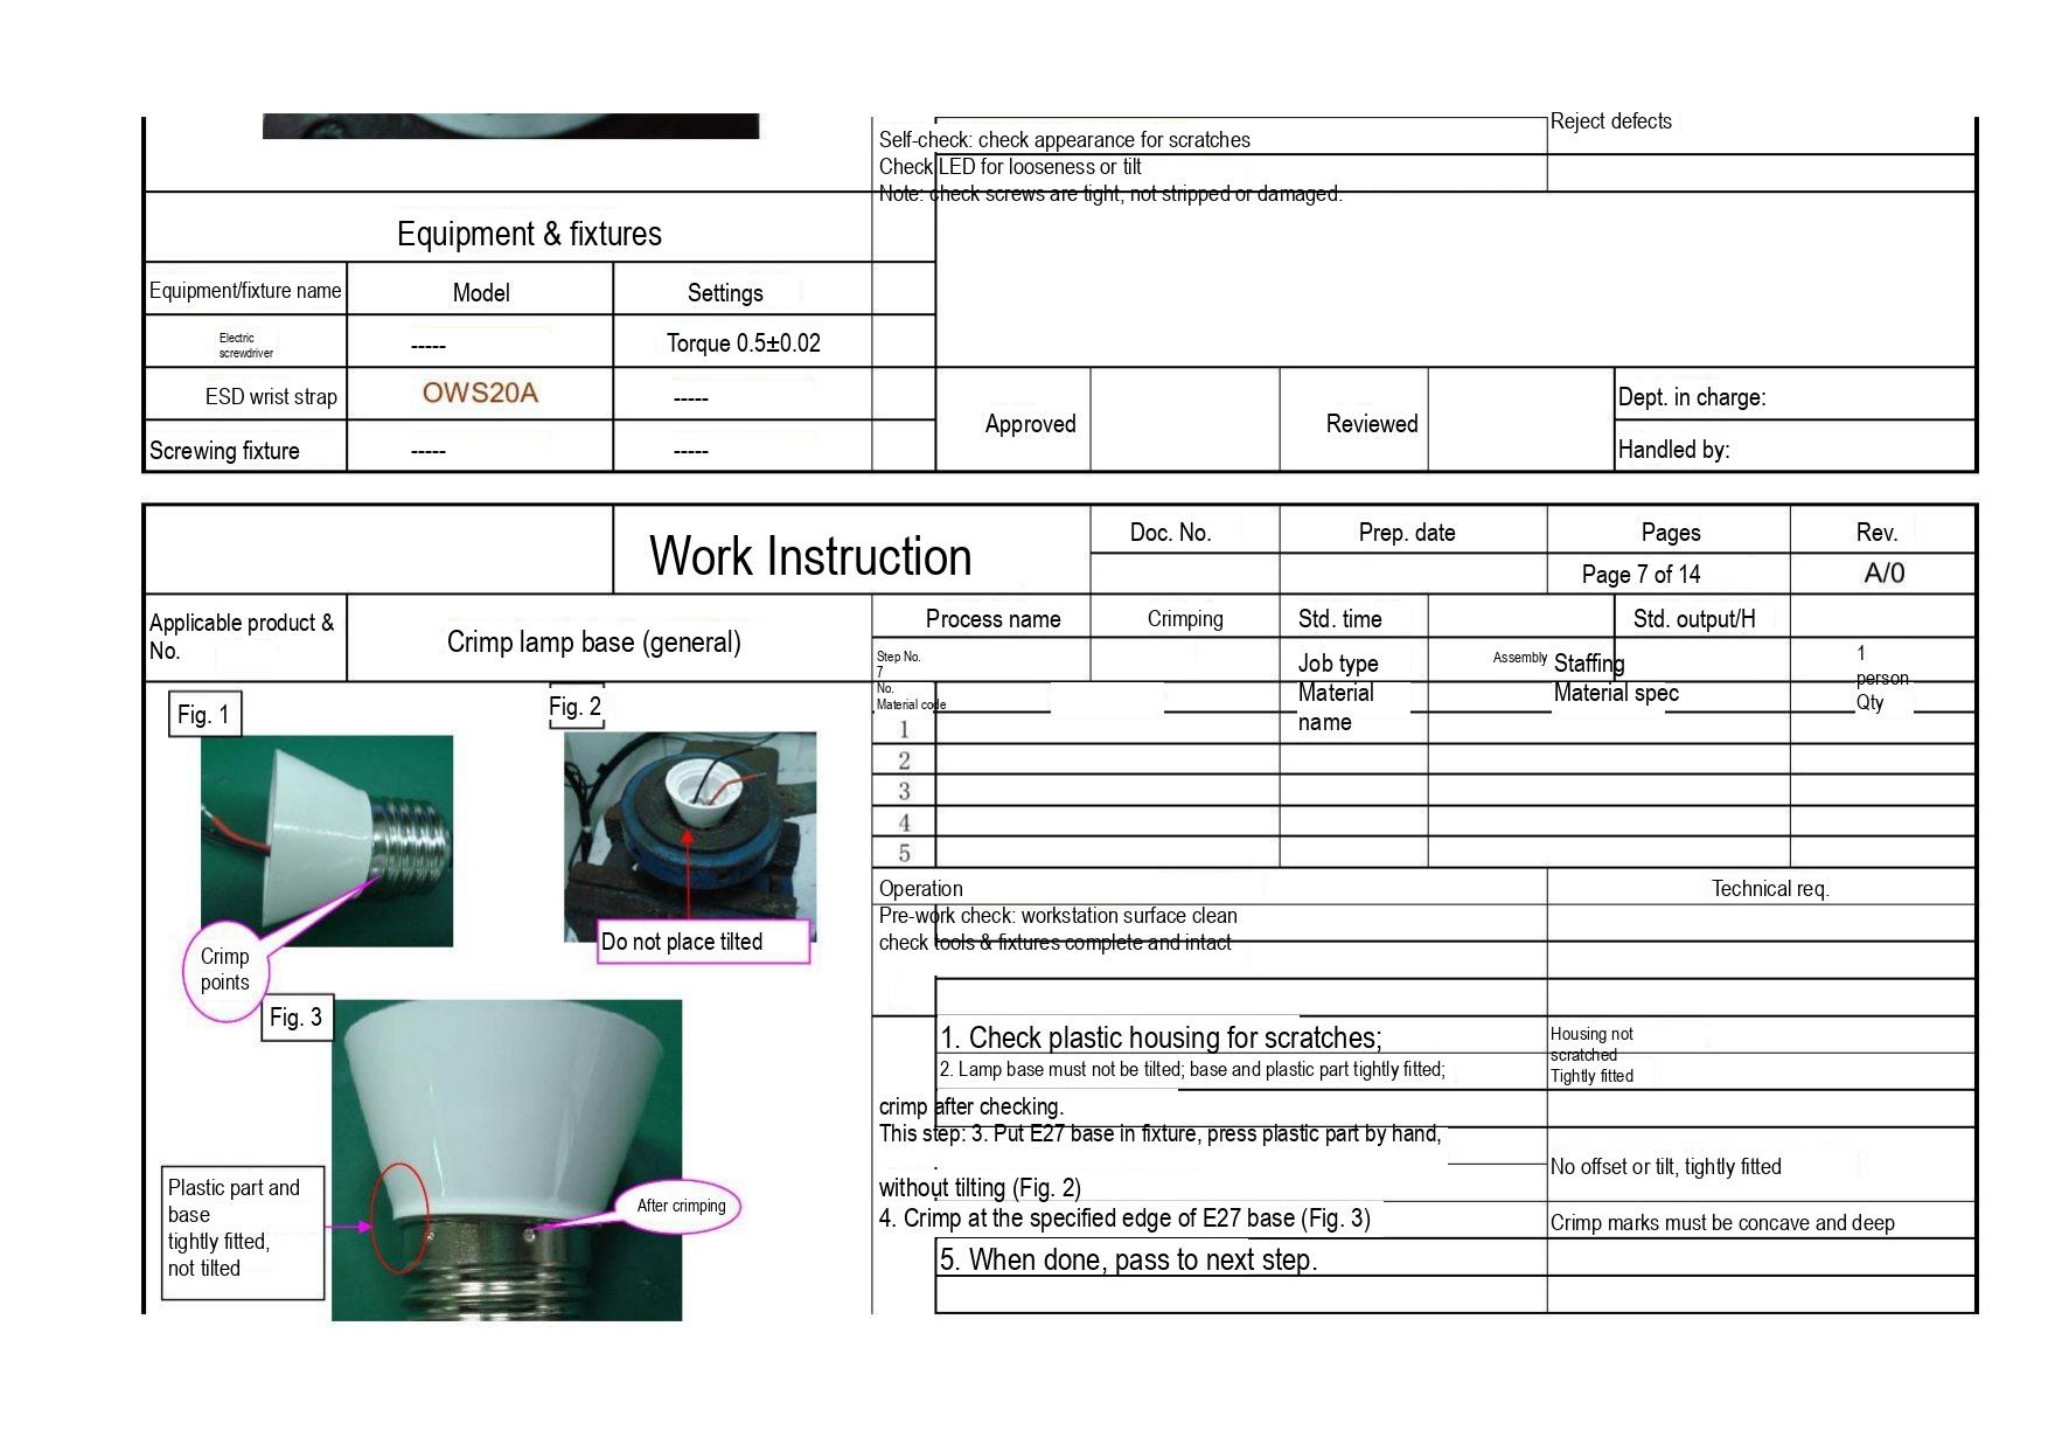Self-check: check appearance for scratches | Reject defects
Check LED for looseness or tilt
Note: check screws are tight, not stripped or damaged.

Equipment & fixtures

| Equipment/fixture name | Model | Settings |
|---|---|---|
| Electric screwdriver | ----- | Torque 0.5±0.02 |
| ESD wrist strap | OWS20A | ----- |
| Screwing fixture | ----- | ----- |

| Approved | | Reviewed | | Dept. in charge: |
|---|---|---|---|---|
| | | | | Handled by: |

| | Work Instruction | Doc. No. | Prep. date | Pages | Rev. |
|---|---|---|---|---|---|
| | | | | Page 7 of 14 | A/0 |

| Applicable product & No. | Crimp lamp base (general) |
|---|---|

| Process name | Crimping | Std. time | | Std. output/H | |
|---|---|---|---|---|---|
| Step No. 7 | | Job type | Assembly | Staffing | 1 person |
| No. | Material code | Material name | | Material spec | Qty |
| 1 | | | | | |
| 2 | | | | | |
| 3 | | | | | |
| 4 | | | | | |
| 5 | | | | | |

Fig. 1
Crimp points

Fig. 2
Do not place tilted

Fig. 3
Plastic part and base tightly fitted, not tilted
After crimping

| Operation | Technical req. |
|---|---|
| Pre-work check: workstation surface clean | |
| check tools & fixtures complete and intact | |
| 1. Check plastic housing for scratches; | Housing not scratched |
| 2. Lamp base must not be tilted; base and plastic part tightly fitted; | Tightly fitted |
| crimp after checking. | |
| This step: 3. Put E27 base in fixture, press plastic part by hand, without tilting (Fig. 2) | No offset or tilt, tightly fitted |
| 4. Crimp at the specified edge of E27 base (Fig. 3) | Crimp marks must be concave and deep |
| 5. When done, pass to next step. | |
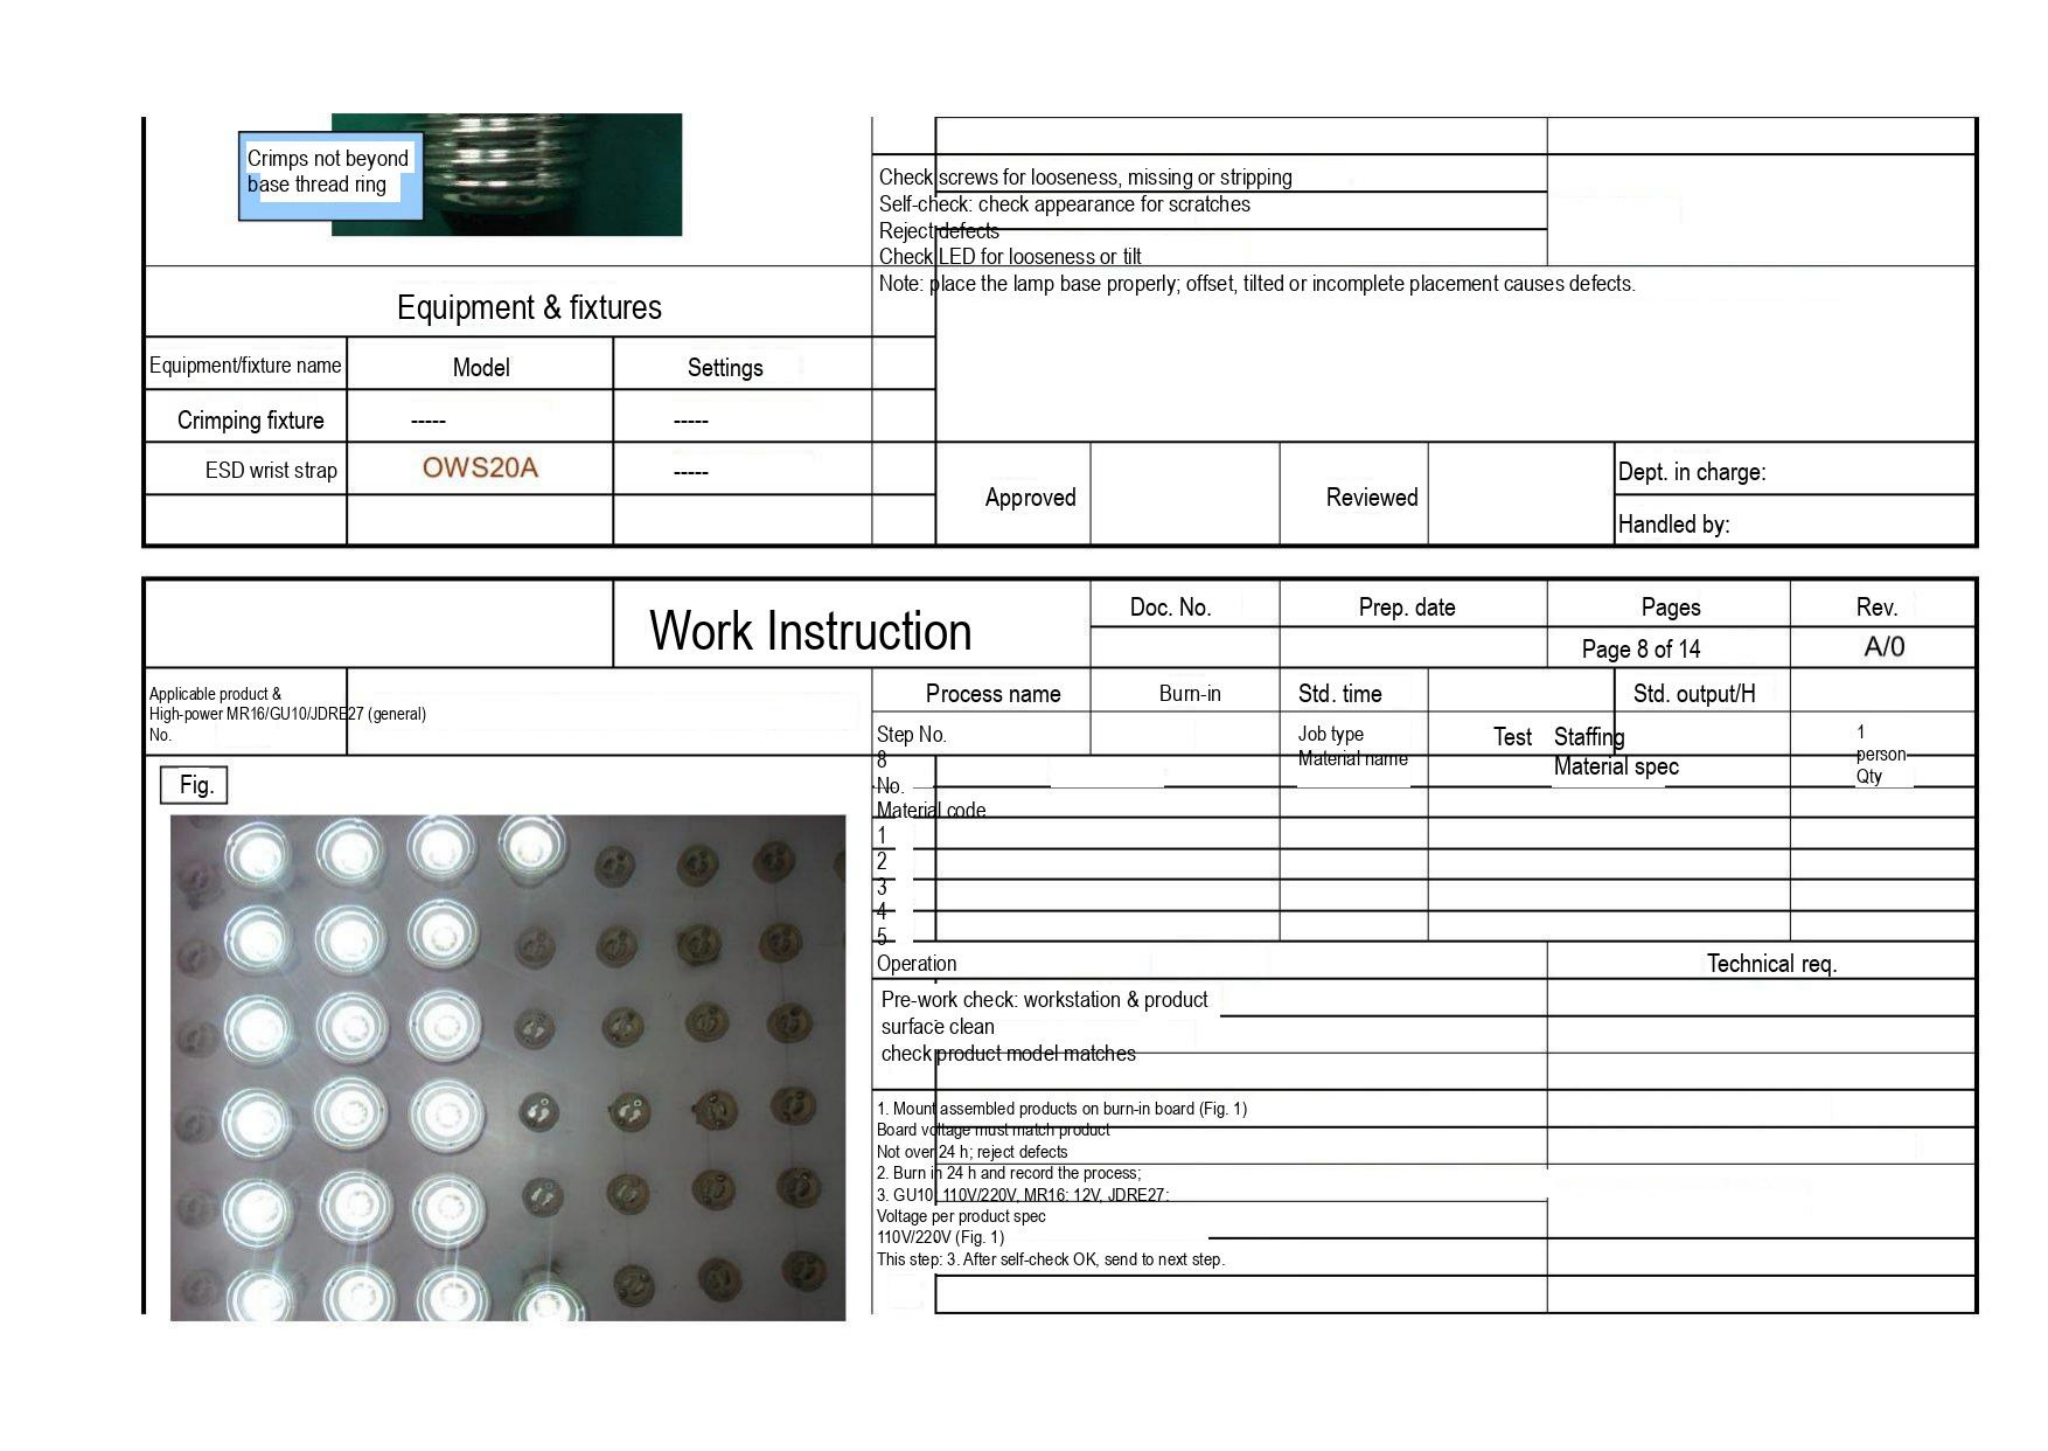Crimps not beyond base thread ring

Check screws for looseness, missing or stripping
Self-check: check appearance for scratches
Reject defects
Check LED for looseness or tilt
Note: place the lamp base properly; offset, tilted or incomplete placement causes defects.

Equipment & fixtures

| Equipment/fixture name | Model | Settings |
|---|---|---|
| Crimping fixture | ----- | ----- |
| ESD wrist strap | OWS20A | ----- |
| | | |

| Approved | | Reviewed | | Dept. in charge: |
|---|---|---|---|---|
| | | | | Handled by: |

| | Work Instruction | Doc. No. | Prep. date | Pages | Rev. |
|---|---|---|---|---|---|
| | | | | Page 8 of 14 | A/0 |

Applicable product & No. High-power MR16/GU10/JDRE27 (general)

| Process name | Burn-in | Std. time | | Std. output/H | |
|---|---|---|---|---|---|
| Step No. 8 | | Job type | Test | Staffing | 1 person |

| No. | Material code | Material name | Material spec | Qty |
|---|---|---|---|---|
| 1 | | | | |
| 2 | | | | |
| 3 | | | | |
| 4 | | | | |
| 5 | | | | |

Fig.

| Operation | Technical req. |
|---|---|
| Pre-work check: workstation & product surface clean check product model matches | |
| 1. Mount assembled products on burn-in board (Fig. 1) Board voltage must match product Not over 24 h; reject defects 2. Burn in 24 h and record the process; 3. GU10 110V/220V, MR16: 12V, JDRE27: Voltage per product spec 110V/220V (Fig. 1) This step: 3. After self-check OK, send to next step. | |
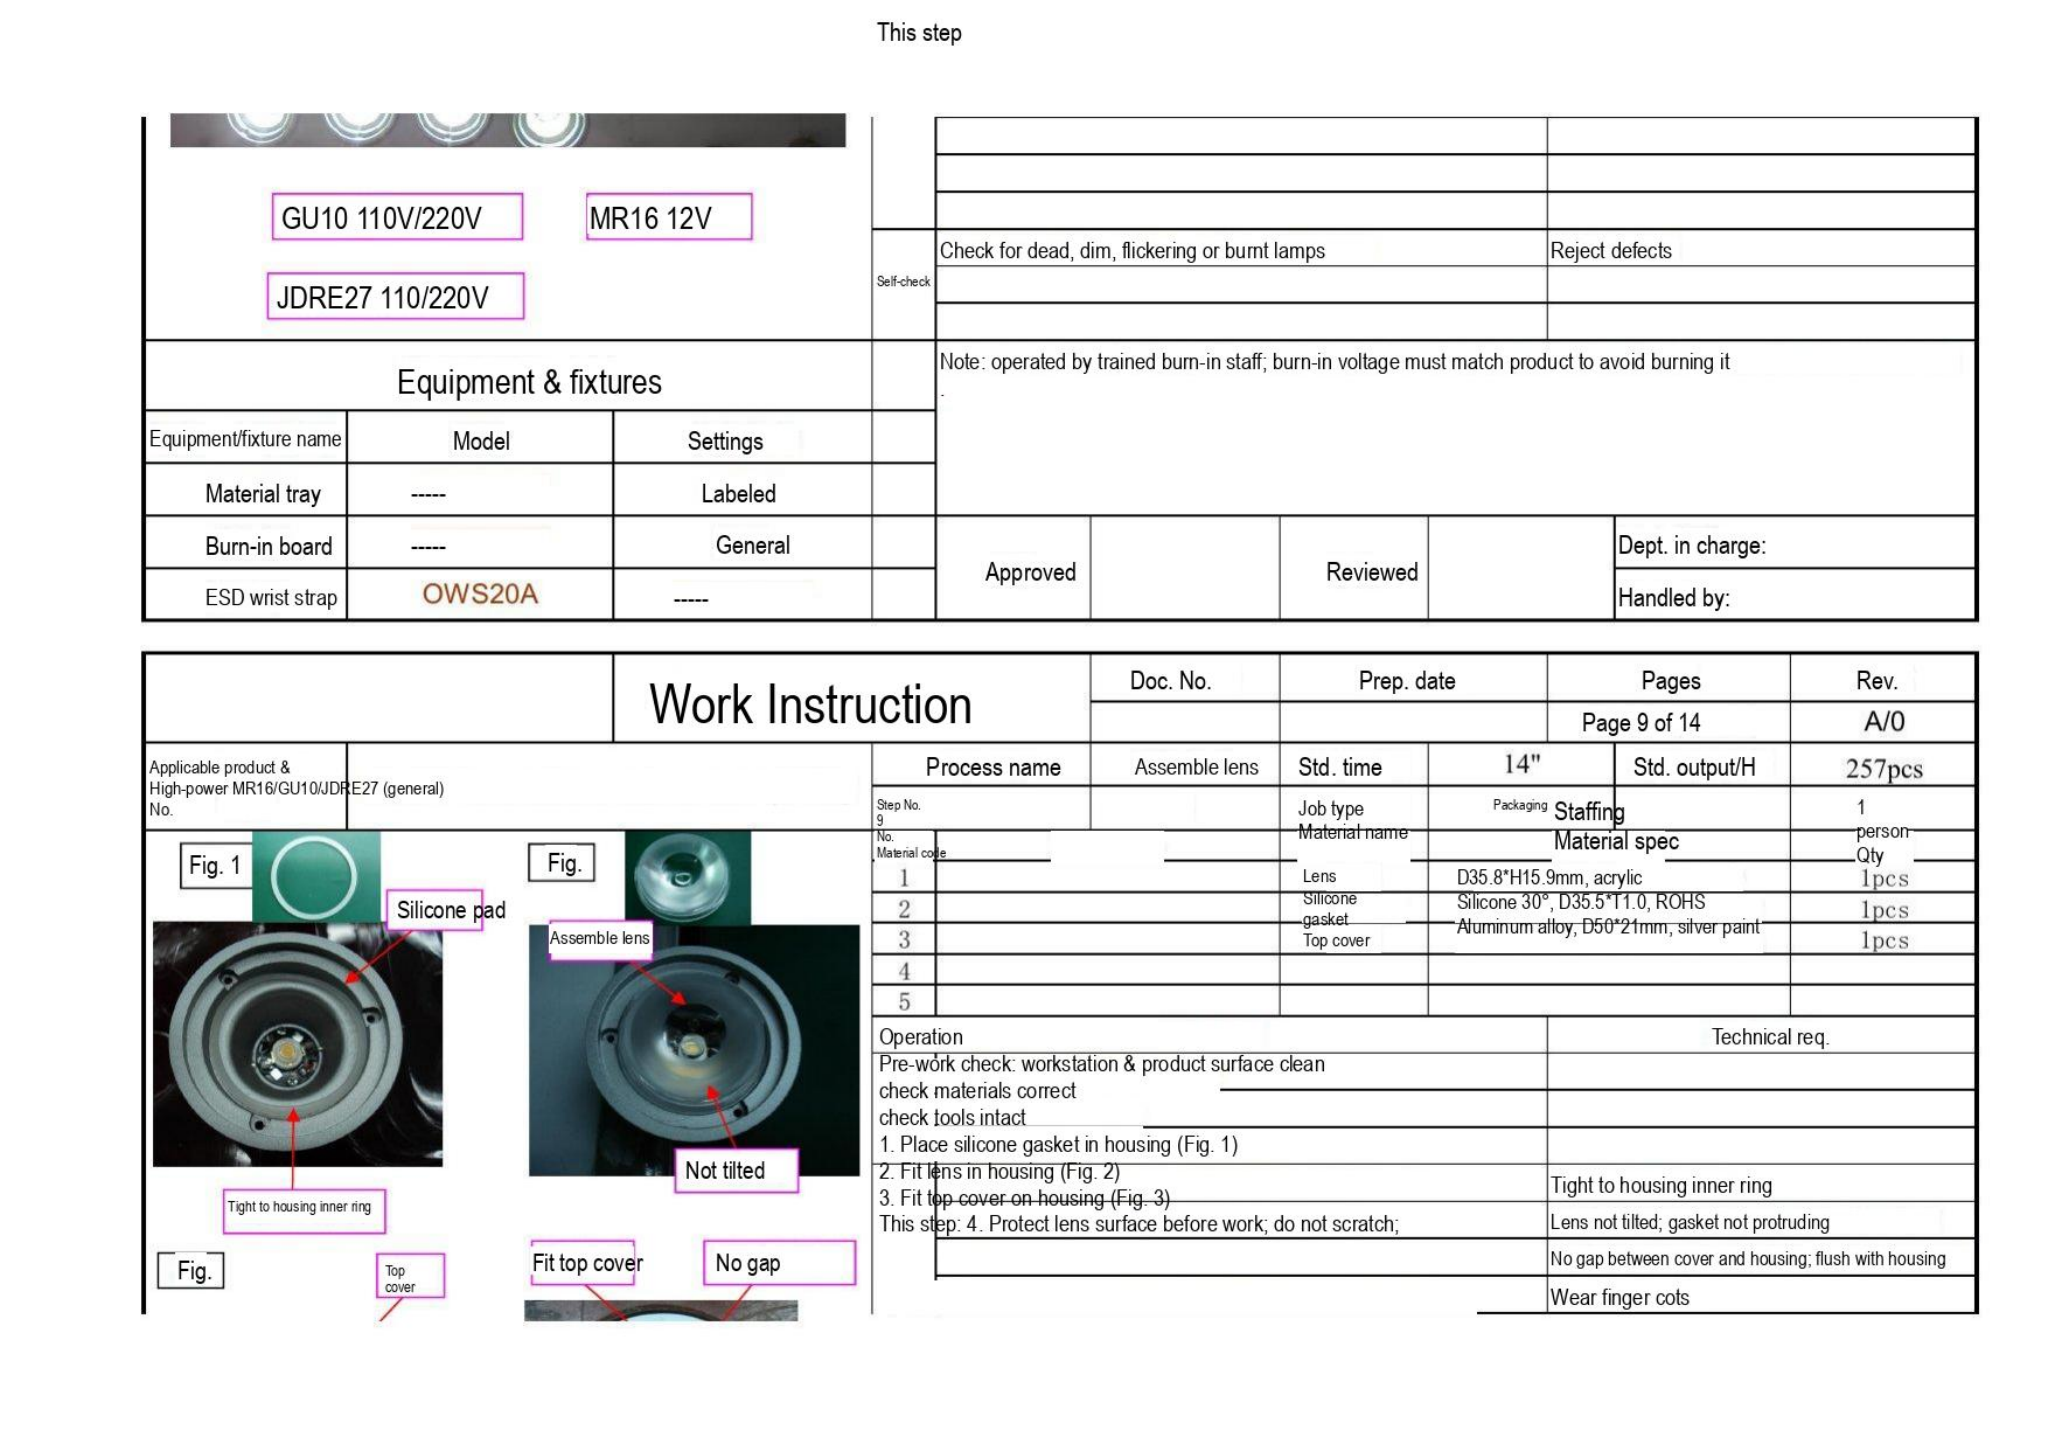This step

GU10 110V/220V

MR16 12V

JDRE27 110/220V

| Self-check | | |
|---|---|---|
| | | |
| | | |
| | | |
| | Check for dead, dim, flickering or burnt lamps | Reject defects |
| | | |
| | | |

Note: operated by trained burn-in staff; burn-in voltage must match product to avoid burning it

**Equipment & fixtures**

| Equipment/fixture name | Model | Settings |
|---|---|---|
| Material tray | ----- | Labeled |
| Burn-in board | ----- | General |
| ESD wrist strap | OWS20A | ----- |

| Approved | | Reviewed | | Dept. in charge: |
|---|---|---|---|---|
| | | | | Handled by: |

**Work Instruction**

| Doc. No. | Prep. date | Pages | Rev. |
|---|---|---|---|
| | | Page 9 of 14 | A/0 |

Applicable product & High-power MR16/GU10/JDRE27 (general)
No.

| Process name | Assemble lens | Std. time | 14" | Std. output/H | 257pcs |
|---|---|---|---|---|---|
| Step No. 9 | | Job type | Packaging | Staffing | 1 person |

| No. | Material code | Material name | Material spec | Qty |
|---|---|---|---|---|
| 1 | | Lens | D35.8*H15.9mm, acrylic | 1pcs |
| 2 | | Silicone gasket | Silicone 30°, D35.5*T1.0, ROHS | 1pcs |
| 3 | | Top cover | Aluminum alloy, D50*21mm, silver paint | 1pcs |
| 4 | | | | |
| 5 | | | | |

| Operation | Technical req. |
|---|---|
| Pre-work check: workstation & product surface clean | |
| check materials correct | |
| check tools intact | |
| 1. Place silicone gasket in housing (Fig. 1) | |
| 2. Fit lens in housing (Fig. 2) | Tight to housing inner ring |
| 3. Fit top cover on housing (Fig. 3) | Lens not tilted; gasket not protruding |
| This step: 4. Protect lens surface before work; do not scratch; | No gap between cover and housing; flush with housing |
| | Wear finger cots |

Fig. 1

Silicone pad

Tight to housing inner ring

Fig.

Assemble lens

Not tilted

Fig.

Top cover

Fit top cover

No gap
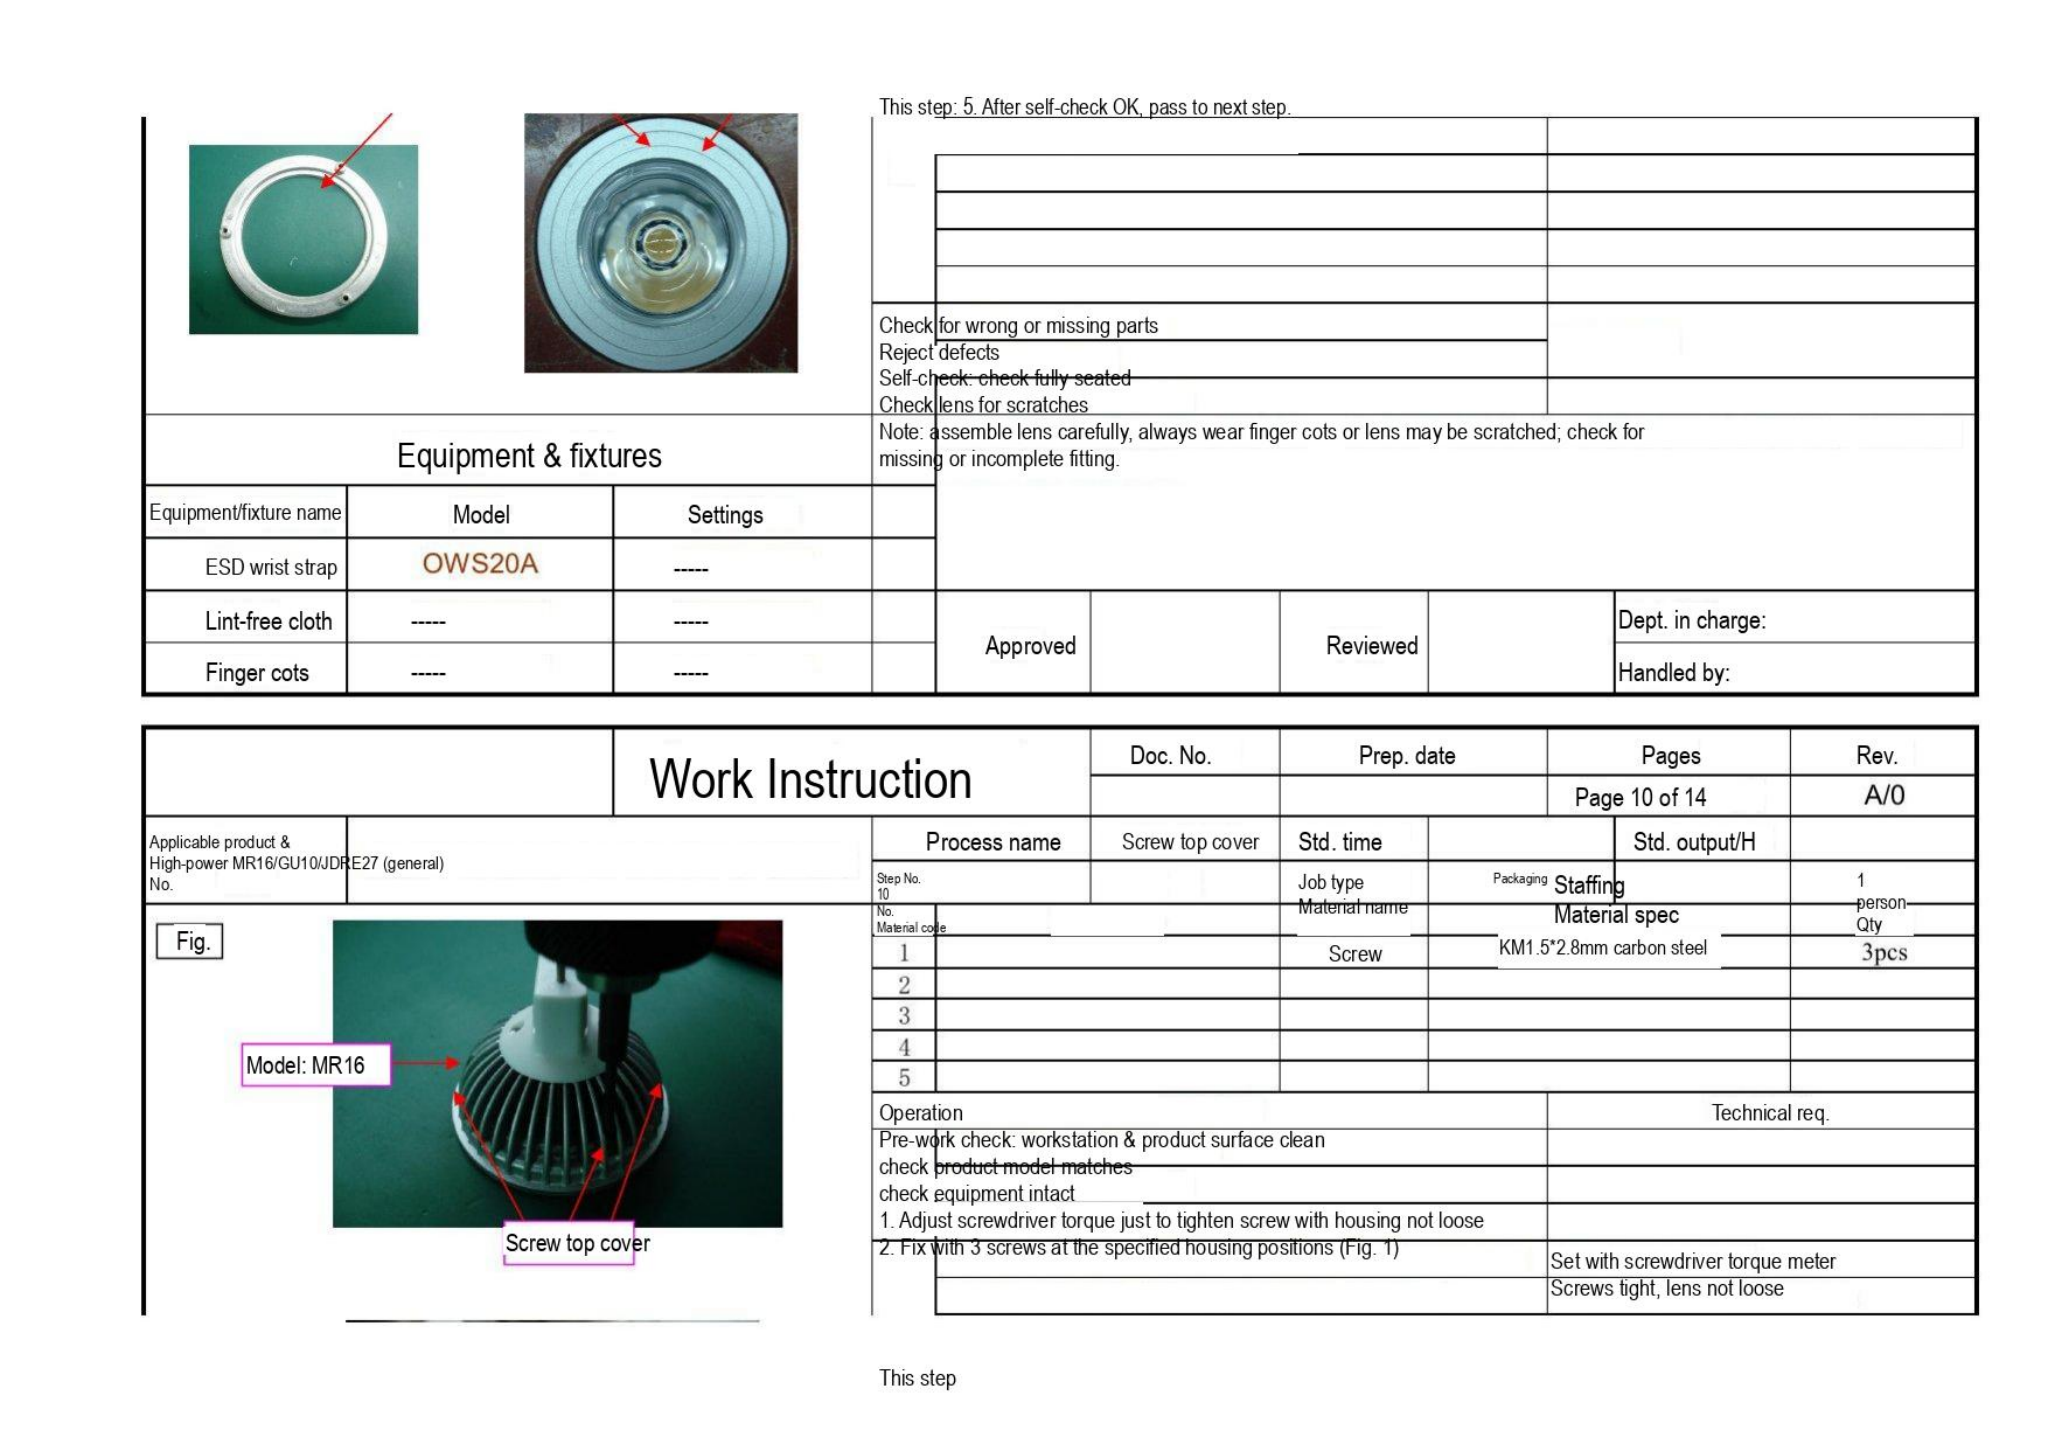This step: 5. After self-check OK, pass to next step.

Check for wrong or missing parts
Reject defects
Self-check: check fully seated
Check lens for scratches
Note: assemble lens carefully, always wear finger cots or lens may be scratched; check for missing or incomplete fitting.

Equipment & fixtures

| Equipment/fixture name | Model | Settings |
|---|---|---|
| ESD wrist strap | OWS20A | ----- |
| Lint-free cloth | ----- | ----- |
| Finger cots | ----- | ----- |

| Approved | | Reviewed | | Dept. in charge: |
|---|---|---|---|---|
| | | | | Handled by: |

Work Instruction

| Doc. No. | Prep. date | Pages | Rev. |
|---|---|---|---|
| | | Page 10 of 14 | A/0 |

Applicable product &
High-power MR16/GU10/JDRE27 (general)
No.

| Process name | Screw top cover | Std. time | | Std. output/H | |
|---|---|---|---|---|---|
| Step No. 10 | | Job type | Packaging | Staffing | 1 person |

| No. | Material code | Material name | Material spec | Qty |
|---|---|---|---|---|
| 1 | | Screw | KM1.5*2.8mm carbon steel | 3pcs |
| 2 | | | | |
| 3 | | | | |
| 4 | | | | |
| 5 | | | | |

Fig.

Model: MR16

Screw top cover

| Operation | Technical req. |
|---|---|
| Pre-work check: workstation & product surface clean | |
| check product model matches | |
| check equipment intact | |
| 1. Adjust screwdriver torque just to tighten screw with housing not loose | Set with screwdriver torque meter |
| 2. Fix with 3 screws at the specified housing positions (Fig. 1) | Screws tight, lens not loose |

This step
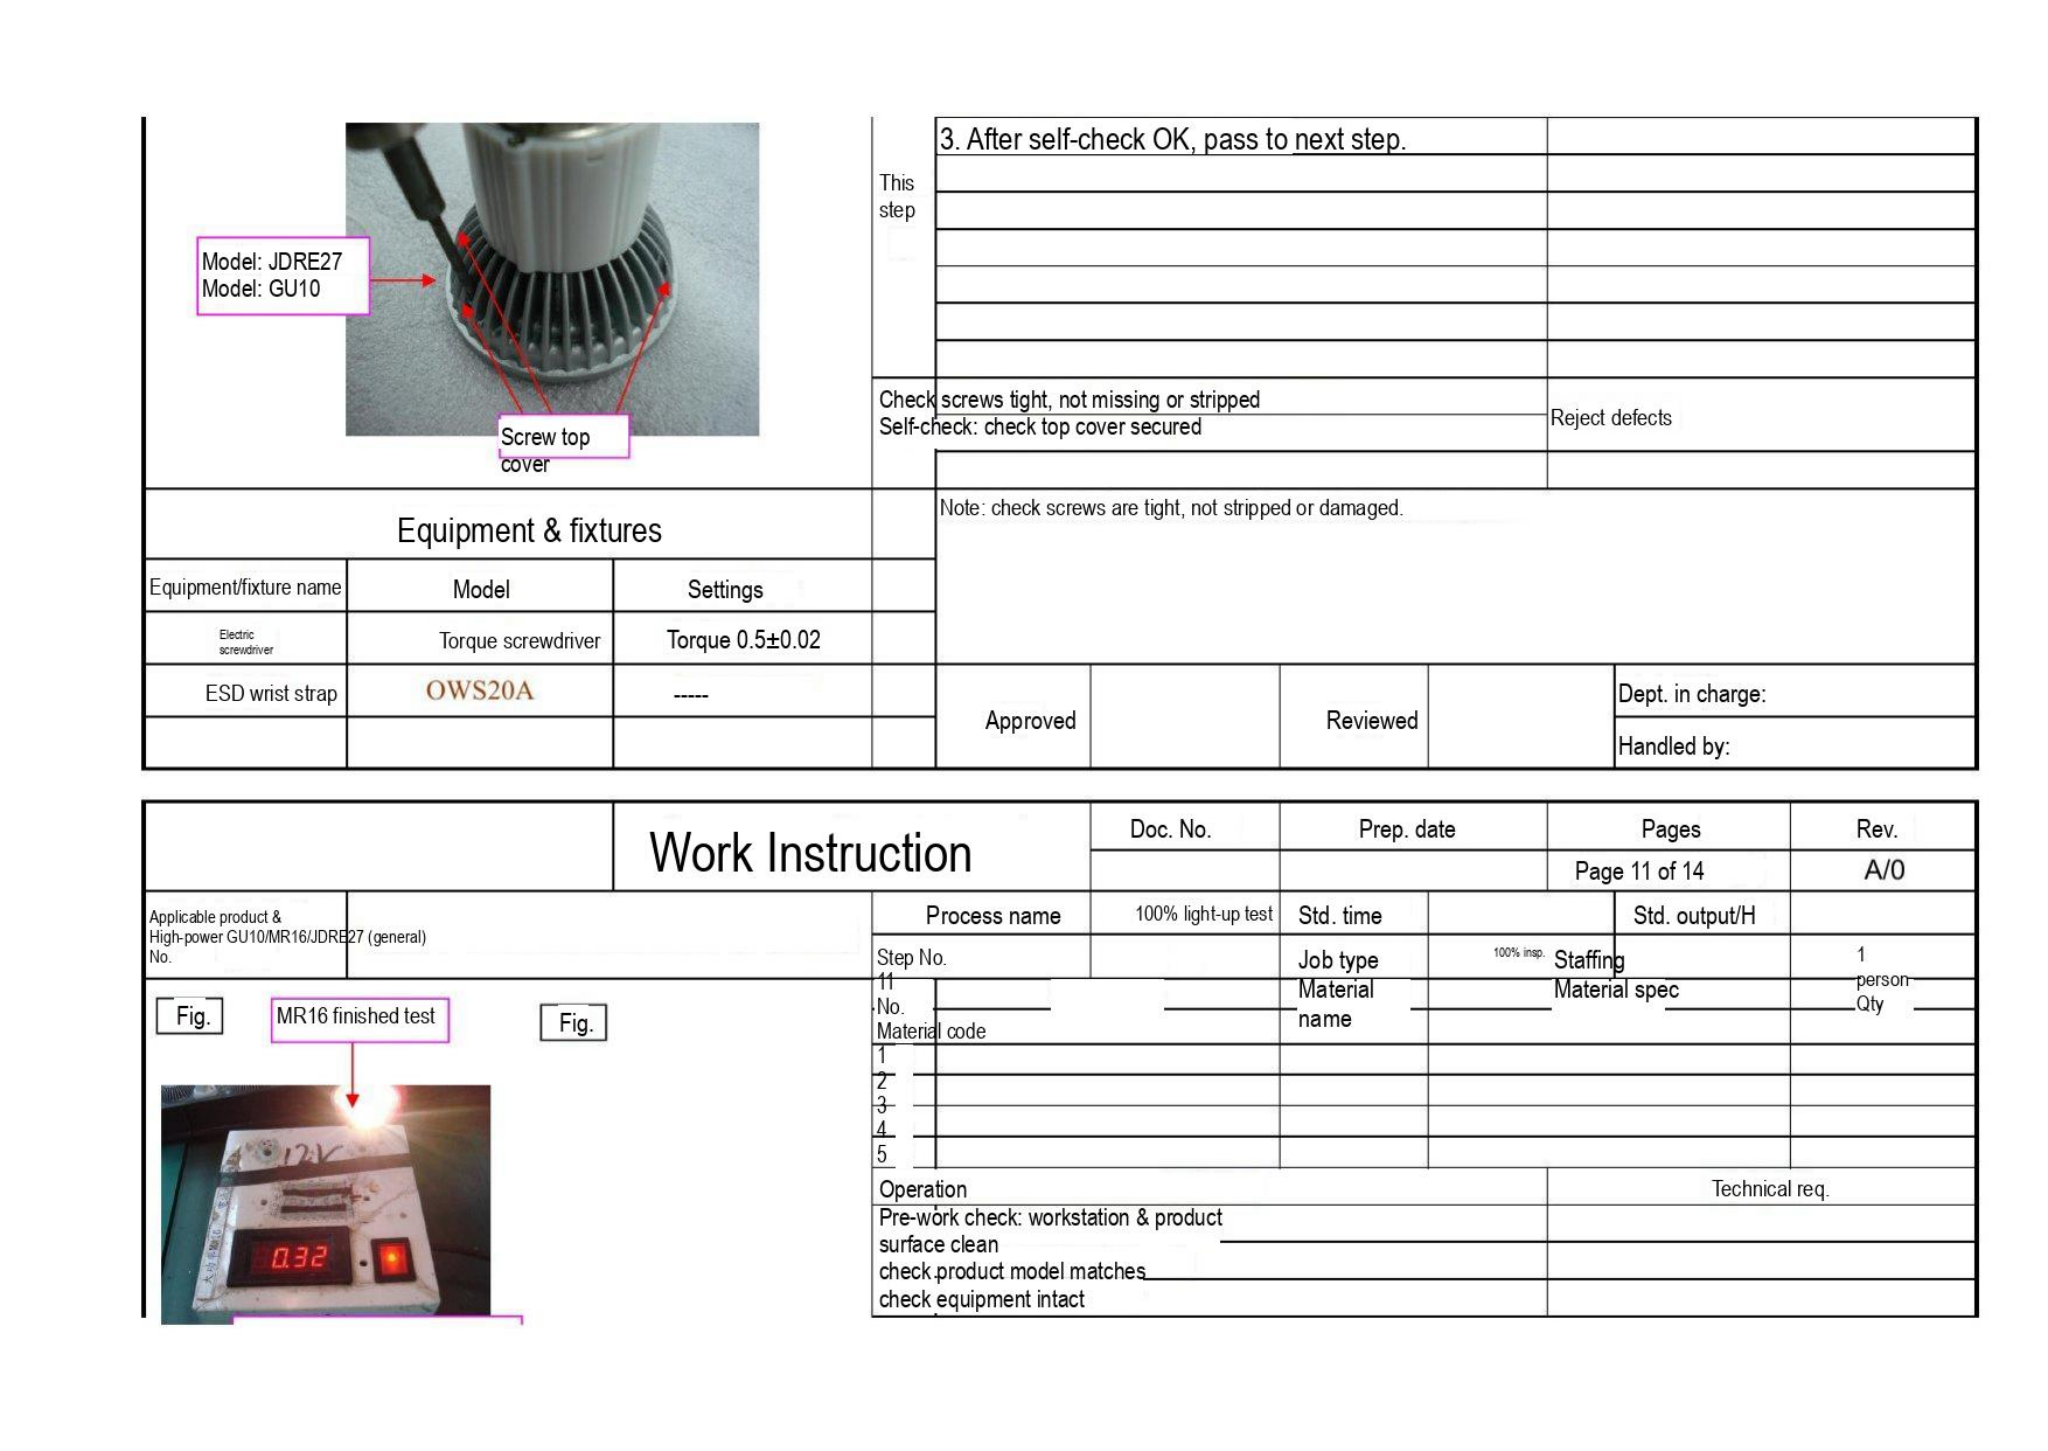Model: JDRE27
Model: GU10

Screw top cover

| This step | 3. After self-check OK, pass to next step. | |
|---|---|---|
| | | |
| | | |
| | | |
| | | |
| | | |
| Check screws tight, not missing or stripped<br>Self-check: check top cover secured | | Reject defects |
| | | |

Note: check screws are tight, not stripped or damaged.

Equipment & fixtures

| Equipment/fixture name | Model | Settings |
|---|---|---|
| Electric screwdriver | Torque screwdriver | Torque 0.5±0.02 |
| ESD wrist strap | OWS20A | ----- |
| | | |

| Approved | | Reviewed | | Dept. in charge: |
|---|---|---|---|---|
| | | | | Handled by: |

| | Work Instruction | Doc. No. | Prep. date | Pages | Rev. |
|---|---|---|---|---|---|
| | | | | Page 11 of 14 | A/0 |

| Applicable product & No. | High-power GU10/MR16/JDRE27 (general) |
|---|---|

| Process name | 100% light-up test | Std. time | | Std. output/H | |
|---|---|---|---|---|---|
| Step No. 11 | | Job type | 100% insp. | Staffing | 1 person |

| No. | Material code | Material name | Material spec | Qty |
|---|---|---|---|---|
| 1 | | | | |
| 2 | | | | |
| 3 | | | | |
| 4 | | | | |
| 5 | | | | |

| Operation | Technical req. |
|---|---|
| Pre-work check: workstation & product | |
| surface clean | |
| check product model matches | |
| check equipment intact | |

Fig.

MR16 finished test

12V

0.32

Fig.
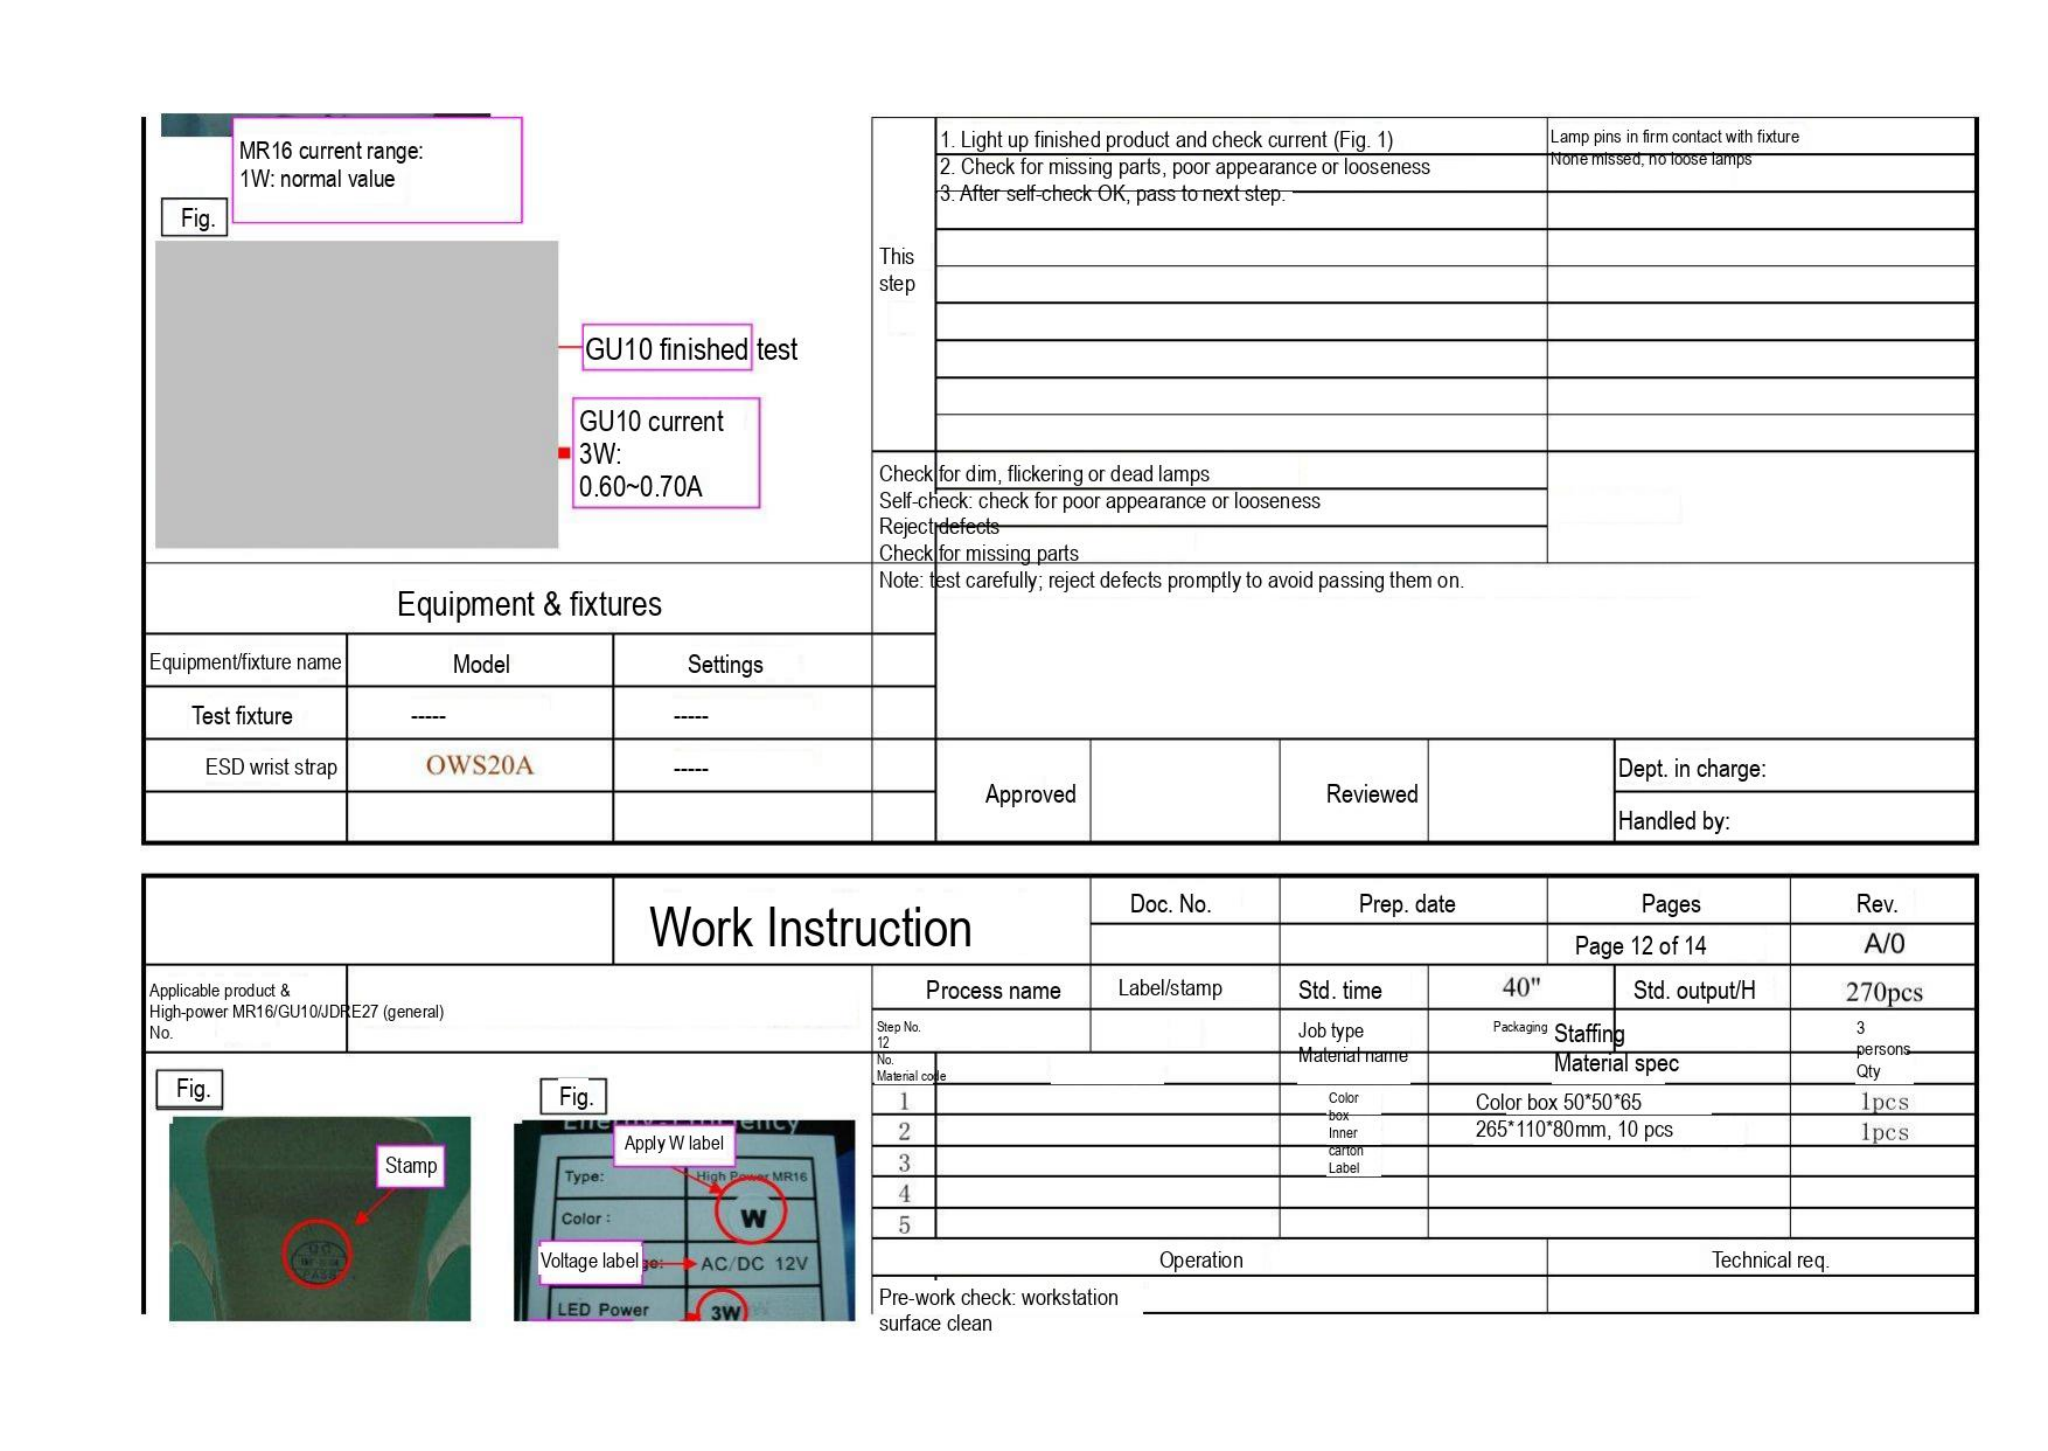MR16 current range:
1W: normal value

Fig.

GU10 finished test

GU10 current
3W:
0.60~0.70A

| This step | 1. Light up finished product and check current (Fig. 1) | Lamp pins in firm contact with fixture |
|---|---|---|
| | 2. Check for missing parts, poor appearance or looseness | None missed, no loose lamps |
| | 3. After self-check OK, pass to next step. | |

Check for dim, flickering or dead lamps
Self-check: check for poor appearance or looseness
Reject defects
Check for missing parts
Note: test carefully; reject defects promptly to avoid passing them on.

Equipment & fixtures

| Equipment/fixture name | Model | Settings |
|---|---|---|
| Test fixture | ----- | ----- |
| ESD wrist strap | OWS20A | ----- |
| | | |

| Approved | | Reviewed | | Dept. in charge: |
|---|---|---|---|---|
| | | | | Handled by: |

Work Instruction

| Doc. No. | Prep. date | Pages | Rev. |
|---|---|---|---|
| | | Page 12 of 14 | A/0 |

Applicable product & No.
High-power MR16/GU10/JDRE27 (general)

| Process name | Label/stamp | Std. time | 40" | Std. output/H | 270pcs |
|---|---|---|---|---|---|
| Step No. 12 | | Job type | Packaging | Staffing | 3 persons |
| No. | Material code | Material name | | Material spec | Qty |
| 1 | | Color box | | Color box 50\*50\*65 | 1pcs |
| 2 | | Inner carton | | 265\*110\*80mm, 10 pcs | 1pcs |
| 3 | | Label | | | |
| 4 | | | | | |
| 5 | | | | | |

| Operation | Technical req. |
|---|---|
| Pre-work check: workstation surface clean | |

Fig.
Stamp

Fig.
Apply W label
Type:
High Power MR16
W
Color:
Voltage label
AC/DC 12V
LED Power
3W